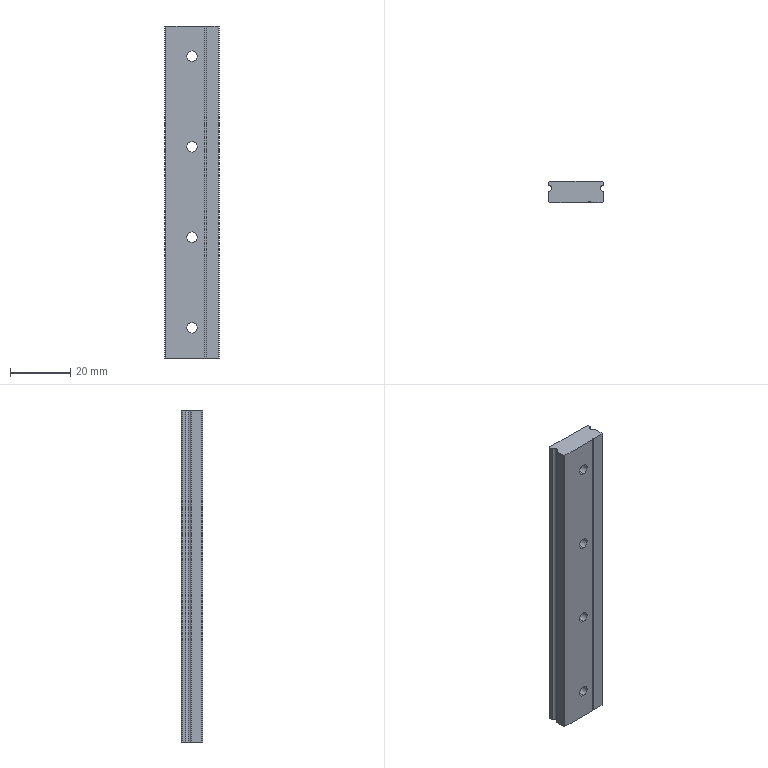Part | SolidWorks | features Extrusion 1, HoleWzd 1, ICE 1, LPattern 1 | 1 solid | 141 faces | box 18 x 7 x 110 mm | volume 12871 mm3 | plane 103 | cylinder 20 | spline 18 | commonest cylinder face diameters 3.5 x8 6 x8 2 x3 0.6 x1